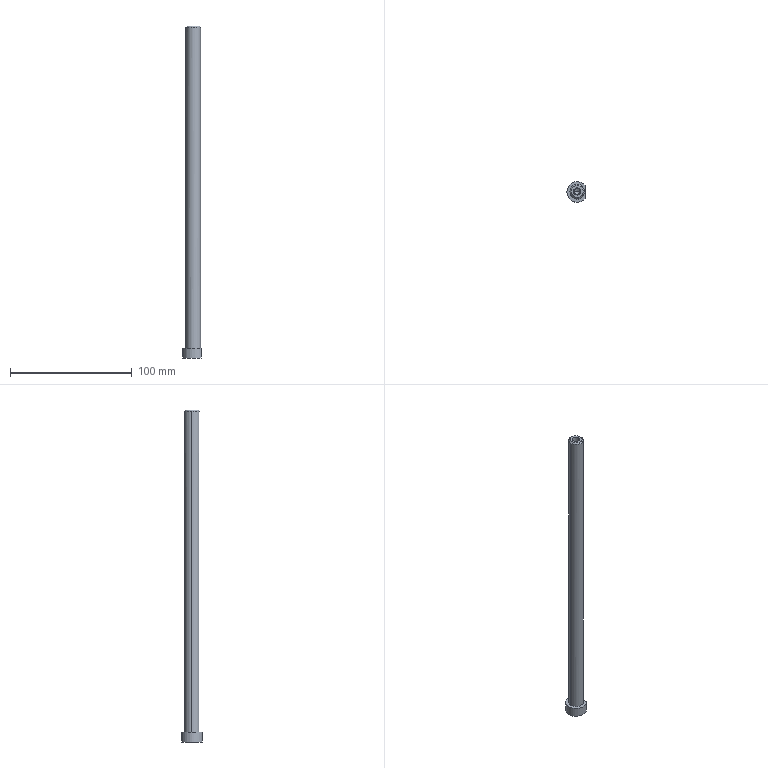Part | Creo | 1 solid | 16 faces | box 15 x 17 x 273 mm | volume 31161 mm3 | cylinder 7 | plane 5 | cone 4 | commonest cylinder face diameters 5 x2 6 x2 12 x2 17 x1
STEP:
#1=CARTESIAN_POINT('',(31.5,12.523,-288.));
#2=VERTEX_POINT('',#1);
#3=CARTESIAN_POINT('',(31.5,23.477,-288.));
#4=VERTEX_POINT('',#3);
#5=CARTESIAN_POINT('',(31.5,12.523,-288.));
#6=DIRECTION('',(0.,1.,0.));
#7=VECTOR('',#6,10.954);
#8=LINE('',#5,#7);
#9=EDGE_CURVE('',#2,#4,#8,.T.);
#10=ORIENTED_EDGE('',*,*,#9,.F.);
#11=CARTESIAN_POINT('',(25.,18.,-288.));
#12=DIRECTION('',(0.,0.,1.));
#13=DIRECTION('',(0.7647,0.6444,0.));
#14=AXIS2_PLACEMENT_3D('',#11,#12,#13);
#15=CIRCLE('',#14,8.5);
#16=EDGE_CURVE('',#4,#2,#15,.T.);
#17=ORIENTED_EDGE('',*,*,#16,.F.);
#18=EDGE_LOOP('',(#10,#17));
#19=FACE_OUTER_BOUND('',#18,.F.);
#20=CARTESIAN_POINT('',(19.,18.,-288.));
#21=VERTEX_POINT('',#20);
#22=CARTESIAN_POINT('',(31.,18.,-288.));
#23=VERTEX_POINT('',#22);
#24=CARTESIAN_POINT('',(25.,18.,-288.));
#25=DIRECTION('',(0.,0.,-1.));
#26=DIRECTION('',(-1.,0.,0.));
#27=AXIS2_PLACEMENT_3D('',#24,#25,#26);
#28=CIRCLE('',#27,6.);
#29=EDGE_CURVE('',#21,#23,#28,.T.);
#30=ORIENTED_EDGE('',*,*,#29,.F.);
#31=CARTESIAN_POINT('',(25.,18.,-288.));
#32=DIRECTION('',(0.,0.,-1.));
#33=DIRECTION('',(1.,0.,0.));
#34=AXIS2_PLACEMENT_3D('',#31,#32,#33);
#35=CIRCLE('',#34,6.);
#36=EDGE_CURVE('',#23,#21,#35,.T.);
#37=ORIENTED_EDGE('',*,*,#36,.F.);
#38=EDGE_LOOP('',(#30,#37));
#39=FACE_BOUND('',#38,.F.);
#40=CARTESIAN_POINT('',(25.,18.,-288.));
#41=DIRECTION('',(0.,0.,1.));
#42=DIRECTION('',(-1.,0.,0.));
#43=AXIS2_PLACEMENT_3D('',#40,#41,#42);
#44=PLANE('',#43);
#45=ADVANCED_FACE('',(#19,#39),#44,.T.);
#46=CARTESIAN_POINT('',(31.5,12.523,-296.));
#47=VERTEX_POINT('',#46);
#48=CARTESIAN_POINT('',(31.5,12.523,-296.));
#49=DIRECTION('',(0.,0.,1.));
#50=VECTOR('',#49,8.);
#51=LINE('',#48,#50);
#52=EDGE_CURVE('',#47,#2,#51,.T.);
#53=ORIENTED_EDGE('',*,*,#52,.T.);
#54=ORIENTED_EDGE('',*,*,#9,.T.);
#55=CARTESIAN_POINT('',(31.5,23.477,-296.));
#56=VERTEX_POINT('',#55);
#57=CARTESIAN_POINT('',(31.5,23.477,-288.));
#58=DIRECTION('',(0.,0.,-1.));
#59=VECTOR('',#58,8.);
#60=LINE('',#57,#59);
#61=EDGE_CURVE('',#4,#56,#60,.T.);
#62=ORIENTED_EDGE('',*,*,#61,.T.);
#63=CARTESIAN_POINT('',(31.5,23.477,-296.));
#64=DIRECTION('',(0.,-1.,0.));
#65=VECTOR('',#64,10.954);
#66=LINE('',#63,#65);
#67=EDGE_CURVE('',#56,#47,#66,.T.);
#68=ORIENTED_EDGE('',*,*,#67,.T.);
#69=EDGE_LOOP('',(#53,#54,#62,#68));
#70=FACE_OUTER_BOUND('',#69,.F.);
#71=CARTESIAN_POINT('',(31.5,53.,-297.));
#72=DIRECTION('',(-1.,0.,0.));
#73=DIRECTION('',(0.,0.,-1.));
#74=AXIS2_PLACEMENT_3D('',#71,#72,#73);
#75=PLANE('',#74);
#76=ADVANCED_FACE('',(#70),#75,.F.);
#77=ORIENTED_EDGE('',*,*,#52,.F.);
#78=CARTESIAN_POINT('',(25.,18.,-296.));
#79=DIRECTION('',(0.,0.,-1.));
#80=DIRECTION('',(0.7647,-0.6444,0.));
#81=AXIS2_PLACEMENT_3D('',#78,#79,#80);
#82=CIRCLE('',#81,8.5);
#83=EDGE_CURVE('',#47,#56,#82,.T.);
#84=ORIENTED_EDGE('',*,*,#83,.T.);
#85=ORIENTED_EDGE('',*,*,#61,.F.);
#86=ORIENTED_EDGE('',*,*,#16,.T.);
#87=EDGE_LOOP('',(#77,#84,#85,#86));
#88=FACE_OUTER_BOUND('',#87,.F.);
#89=CARTESIAN_POINT('',(25.,18.,-296.));
#90=DIRECTION('',(0.,0.,1.));
#91=DIRECTION('',(-1.,0.,0.));
#92=AXIS2_PLACEMENT_3D('',#89,#90,#91);
#93=CYLINDRICAL_SURFACE('',#92,8.5);
#94=ADVANCED_FACE('',(#88),#93,.T.);
#95=ORIENTED_EDGE('',*,*,#67,.F.);
#96=ORIENTED_EDGE('',*,*,#83,.F.);
#97=EDGE_LOOP('',(#95,#96));
#98=FACE_OUTER_BOUND('',#97,.F.);
#99=CARTESIAN_POINT('',(25.,18.,-296.));
#100=DIRECTION('',(0.,0.,-1.));
#101=DIRECTION('',(1.,0.,0.));
#102=AXIS2_PLACEMENT_3D('',#99,#100,#101);
#103=PLANE('',#102);
#104=ADVANCED_FACE('',(#98),#103,.T.);
#105=CARTESIAN_POINT('',(25.,24.,-24.));
#106=VERTEX_POINT('',#105);
#107=CARTESIAN_POINT('',(19.,18.,-24.));
#108=VERTEX_POINT('',#107);
#109=CARTESIAN_POINT('',(25.,18.,-24.));
#110=DIRECTION('',(0.,0.,1.));
#111=DIRECTION('',(0.,1.,0.));
#112=AXIS2_PLACEMENT_3D('',#109,#110,#111);
#113=CIRCLE('',#112,6.);
#114=EDGE_CURVE('',#106,#108,#113,.T.);
#115=ORIENTED_EDGE('',*,*,#114,.T.);
#116=CARTESIAN_POINT('',(19.,18.,-288.));
#117=DIRECTION('',(0.,0.,1.));
#118=VECTOR('',#117,264.);
#119=LINE('',#116,#118);
#120=EDGE_CURVE('',#21,#108,#119,.T.);
#121=ORIENTED_EDGE('',*,*,#120,.F.);
#122=ORIENTED_EDGE('',*,*,#29,.T.);
#123=CARTESIAN_POINT('',(31.,18.,-24.));
#124=VERTEX_POINT('',#123);
#125=CARTESIAN_POINT('',(31.,18.,-288.));
#126=DIRECTION('',(0.,0.,1.));
#127=VECTOR('',#126,264.);
#128=LINE('',#125,#127);
#129=EDGE_CURVE('',#23,#124,#128,.T.);
#130=ORIENTED_EDGE('',*,*,#129,.T.);
#131=CARTESIAN_POINT('',(25.,18.,-24.));
#132=DIRECTION('',(0.,0.,1.));
#133=DIRECTION('',(1.,0.,0.));
#134=AXIS2_PLACEMENT_3D('',#131,#132,#133);
#135=CIRCLE('',#134,6.);
#136=EDGE_CURVE('',#124,#106,#135,.T.);
#137=ORIENTED_EDGE('',*,*,#136,.T.);
#138=EDGE_LOOP('',(#115,#121,#122,#130,#137));
#139=FACE_OUTER_BOUND('',#138,.F.);
#140=CARTESIAN_POINT('',(25.,18.,-351.131));
#141=DIRECTION('',(0.,0.,1.));
#142=DIRECTION('',(-1.,0.,0.));
#143=AXIS2_PLACEMENT_3D('',#140,#141,#142);
#144=CYLINDRICAL_SURFACE('',#143,6.);
#145=ADVANCED_FACE('',(#139),#144,.T.);
#146=ORIENTED_EDGE('',*,*,#114,.F.);
#147=CARTESIAN_POINT('',(25.,23.,-23.));
#148=VERTEX_POINT('',#147);
#149=CARTESIAN_POINT('',(25.,23.,-23.));
#150=DIRECTION('',(0.,0.7071,-0.7071));
#151=VECTOR('',#150,1.414);
#152=LINE('',#149,#151);
#153=EDGE_CURVE('',#148,#106,#152,.T.);
#154=ORIENTED_EDGE('',*,*,#153,.F.);
#155=CARTESIAN_POINT('',(25.,13.,-23.));
#156=VERTEX_POINT('',#155);
#157=CARTESIAN_POINT('',(25.,18.,-23.));
#158=DIRECTION('',(0.,0.,1.));
#159=DIRECTION('',(0.,1.,0.));
#160=AXIS2_PLACEMENT_3D('',#157,#158,#159);
#161=CIRCLE('',#160,5.);
#162=EDGE_CURVE('',#148,#156,#161,.T.);
#163=ORIENTED_EDGE('',*,*,#162,.T.);
#164=CARTESIAN_POINT('',(25.,12.,-24.));
#165=VERTEX_POINT('',#164);
#166=CARTESIAN_POINT('',(25.,13.,-23.));
#167=DIRECTION('',(0.,-0.7071,-0.7071));
#168=VECTOR('',#167,1.414);
#169=LINE('',#166,#168);
#170=EDGE_CURVE('',#156,#165,#169,.T.);
#171=ORIENTED_EDGE('',*,*,#170,.T.);
#172=CARTESIAN_POINT('',(25.,18.,-24.));
#173=DIRECTION('',(0.,0.,1.));
#174=DIRECTION('',(-1.,0.,0.));
#175=AXIS2_PLACEMENT_3D('',#172,#173,#174);
#176=CIRCLE('',#175,6.);
#177=EDGE_CURVE('',#108,#165,#176,.T.);
#178=ORIENTED_EDGE('',*,*,#177,.F.);
#179=EDGE_LOOP('',(#146,#154,#163,#171,#178));
#180=FACE_OUTER_BOUND('',#179,.F.);
#181=CARTESIAN_POINT('',(25.,18.,-23.5));
#182=DIRECTION('',(0.,0.,-1.));
#183=DIRECTION('',(0.,1.,0.));
#184=AXIS2_PLACEMENT_3D('',#181,#182,#183);
#185=CONICAL_SURFACE('',#184,5.5,45.);
#186=ADVANCED_FACE('',(#180),#185,.T.);
#187=CARTESIAN_POINT('',(25.,18.,-24.));
#188=DIRECTION('',(0.,0.,1.));
#189=DIRECTION('',(0.,-1.,0.));
#190=AXIS2_PLACEMENT_3D('',#187,#188,#189);
#191=CIRCLE('',#190,6.);
#192=EDGE_CURVE('',#165,#124,#191,.T.);
#193=ORIENTED_EDGE('',*,*,#192,.F.);
#194=ORIENTED_EDGE('',*,*,#170,.F.);
#195=CARTESIAN_POINT('',(25.,18.,-23.));
#196=DIRECTION('',(0.,0.,1.));
#197=DIRECTION('',(0.,-1.,0.));
#198=AXIS2_PLACEMENT_3D('',#195,#196,#197);
#199=CIRCLE('',#198,5.);
#200=EDGE_CURVE('',#156,#148,#199,.T.);
#201=ORIENTED_EDGE('',*,*,#200,.T.);
#202=ORIENTED_EDGE('',*,*,#153,.T.);
#203=ORIENTED_EDGE('',*,*,#136,.F.);
#204=EDGE_LOOP('',(#193,#194,#201,#202,#203));
#205=FACE_OUTER_BOUND('',#204,.F.);
#206=CARTESIAN_POINT('',(25.,18.,-23.5));
#207=DIRECTION('',(0.,0.,-1.));
#208=DIRECTION('',(0.,1.,0.));
#209=AXIS2_PLACEMENT_3D('',#206,#207,#208);
#210=CONICAL_SURFACE('',#209,5.5,45.);
#211=ADVANCED_FACE('',(#205),#210,.T.);
#212=ORIENTED_EDGE('',*,*,#177,.T.);
#213=ORIENTED_EDGE('',*,*,#192,.T.);
#214=ORIENTED_EDGE('',*,*,#129,.F.);
#215=ORIENTED_EDGE('',*,*,#36,.T.);
#216=ORIENTED_EDGE('',*,*,#120,.T.);
#217=EDGE_LOOP('',(#212,#213,#214,#215,#216));
#218=FACE_OUTER_BOUND('',#217,.F.);
#219=CARTESIAN_POINT('',(25.,18.,-351.131));
#220=DIRECTION('',(0.,0.,1.));
#221=DIRECTION('',(-1.,0.,0.));
#222=AXIS2_PLACEMENT_3D('',#219,#220,#221);
#223=CYLINDRICAL_SURFACE('',#222,6.);
#224=ADVANCED_FACE('',(#218),#223,.T.);
#225=ORIENTED_EDGE('',*,*,#200,.F.);
#226=ORIENTED_EDGE('',*,*,#162,.F.);
#227=EDGE_LOOP('',(#225,#226));
#228=FACE_OUTER_BOUND('',#227,.F.);
#229=CARTESIAN_POINT('',(25.,15.,-23.));
#230=VERTEX_POINT('',#229);
#231=CARTESIAN_POINT('',(22.,18.,-23.));
#232=VERTEX_POINT('',#231);
#233=CARTESIAN_POINT('',(25.,18.,-23.));
#234=DIRECTION('',(0.,0.,-1.));
#235=DIRECTION('',(0.,-1.,0.));
#236=AXIS2_PLACEMENT_3D('',#233,#234,#235);
#237=CIRCLE('',#236,3.);
#238=EDGE_CURVE('',#230,#232,#237,.T.);
#239=ORIENTED_EDGE('',*,*,#238,.F.);
#240=CARTESIAN_POINT('',(28.,18.,-23.));
#241=VERTEX_POINT('',#240);
#242=CARTESIAN_POINT('',(25.,18.,-23.));
#243=DIRECTION('',(0.,0.,-1.));
#244=DIRECTION('',(1.,0.,0.));
#245=AXIS2_PLACEMENT_3D('',#242,#243,#244);
#246=CIRCLE('',#245,3.);
#247=EDGE_CURVE('',#241,#230,#246,.T.);
#248=ORIENTED_EDGE('',*,*,#247,.F.);
#249=CARTESIAN_POINT('',(25.,18.,-23.));
#250=DIRECTION('',(0.,0.,-1.));
#251=DIRECTION('',(-1.,0.,0.));
#252=AXIS2_PLACEMENT_3D('',#249,#250,#251);
#253=CIRCLE('',#252,3.);
#254=EDGE_CURVE('',#232,#241,#253,.T.);
#255=ORIENTED_EDGE('',*,*,#254,.F.);
#256=EDGE_LOOP('',(#239,#248,#255));
#257=FACE_BOUND('',#256,.F.);
#258=CARTESIAN_POINT('',(-50.,35.,-23.));
#259=DIRECTION('',(0.,0.,1.));
#260=DIRECTION('',(-1.,0.,0.));
#261=AXIS2_PLACEMENT_3D('',#258,#259,#260);
#262=PLANE('',#261);
#263=ADVANCED_FACE('',(#228,#257),#262,.T.);
#264=CARTESIAN_POINT('',(22.,18.,-38.872));
#265=VERTEX_POINT('',#264);
#266=CARTESIAN_POINT('',(28.,18.,-38.872));
#267=VERTEX_POINT('',#266);
#268=CARTESIAN_POINT('',(25.,18.,-38.872));
#269=DIRECTION('',(0.,0.,1.));
#270=DIRECTION('',(-1.,0.,0.));
#271=AXIS2_PLACEMENT_3D('',#268,#269,#270);
#272=CIRCLE('',#271,3.);
#273=EDGE_CURVE('',#265,#267,#272,.T.);
#274=ORIENTED_EDGE('',*,*,#273,.T.);
#275=CARTESIAN_POINT('',(28.,18.,-23.));
#276=DIRECTION('',(0.,0.,-1.));
#277=VECTOR('',#276,15.872);
#278=LINE('',#275,#277);
#279=EDGE_CURVE('',#241,#267,#278,.T.);
#280=ORIENTED_EDGE('',*,*,#279,.F.);
#281=ORIENTED_EDGE('',*,*,#247,.T.);
#282=ORIENTED_EDGE('',*,*,#238,.T.);
#283=CARTESIAN_POINT('',(22.,18.,-23.));
#284=DIRECTION('',(0.,0.,-1.));
#285=VECTOR('',#284,15.872);
#286=LINE('',#283,#285);
#287=EDGE_CURVE('',#232,#265,#286,.T.);
#288=ORIENTED_EDGE('',*,*,#287,.T.);
#289=EDGE_LOOP('',(#274,#280,#281,#282,#288));
#290=FACE_OUTER_BOUND('',#289,.F.);
#291=CARTESIAN_POINT('',(25.,18.,-16.372));
#292=DIRECTION('',(0.,0.,-1.));
#293=DIRECTION('',(1.,0.,0.));
#294=AXIS2_PLACEMENT_3D('',#291,#292,#293);
#295=CYLINDRICAL_SURFACE('',#294,3.);
#296=ADVANCED_FACE('',(#290),#295,.F.);
#297=CARTESIAN_POINT('',(25.,18.,-38.872));
#298=DIRECTION('',(0.,0.,1.));
#299=DIRECTION('',(1.,0.,0.));
#300=AXIS2_PLACEMENT_3D('',#297,#298,#299);
#301=CIRCLE('',#300,3.);
#302=EDGE_CURVE('',#267,#265,#301,.T.);
#303=ORIENTED_EDGE('',*,*,#302,.F.);
#304=ORIENTED_EDGE('',*,*,#273,.F.);
#305=EDGE_LOOP('',(#303,#304));
#306=FACE_OUTER_BOUND('',#305,.F.);
#307=CARTESIAN_POINT('',(27.5,18.,-38.872));
#308=VERTEX_POINT('',#307);
#309=CARTESIAN_POINT('',(22.5,18.,-38.872));
#310=VERTEX_POINT('',#309);
#311=CARTESIAN_POINT('',(25.,18.,-38.872));
#312=DIRECTION('',(0.,0.,-1.));
#313=DIRECTION('',(1.,0.,0.));
#314=AXIS2_PLACEMENT_3D('',#311,#312,#313);
#315=CIRCLE('',#314,2.5);
#316=EDGE_CURVE('',#308,#310,#315,.T.);
#317=ORIENTED_EDGE('',*,*,#316,.F.);
#318=CARTESIAN_POINT('',(25.,18.,-38.872));
#319=DIRECTION('',(0.,0.,-1.));
#320=DIRECTION('',(-1.,0.,0.));
#321=AXIS2_PLACEMENT_3D('',#318,#319,#320);
#322=CIRCLE('',#321,2.5);
#323=EDGE_CURVE('',#310,#308,#322,.T.);
#324=ORIENTED_EDGE('',*,*,#323,.F.);
#325=EDGE_LOOP('',(#317,#324));
#326=FACE_BOUND('',#325,.F.);
#327=CARTESIAN_POINT('',(25.,18.,-38.872));
#328=DIRECTION('',(0.,0.,-1.));
#329=DIRECTION('',(1.,0.,0.));
#330=AXIS2_PLACEMENT_3D('',#327,#328,#329);
#331=PLANE('',#330);
#332=ADVANCED_FACE('',(#306,#326),#331,.F.);
#333=ORIENTED_EDGE('',*,*,#316,.T.);
#334=CARTESIAN_POINT('',(22.5,18.,-40.342));
#335=VERTEX_POINT('',#334);
#336=CARTESIAN_POINT('',(22.5,18.,-38.872));
#337=DIRECTION('',(0.,0.,-1.));
#338=VECTOR('',#337,1.47);
#339=LINE('',#336,#338);
#340=EDGE_CURVE('',#310,#335,#339,.T.);
#341=ORIENTED_EDGE('',*,*,#340,.T.);
#342=CARTESIAN_POINT('',(27.5,18.,-40.342));
#343=VERTEX_POINT('',#342);
#344=CARTESIAN_POINT('',(25.,18.,-40.342));
#345=DIRECTION('',(0.,0.,1.));
#346=DIRECTION('',(-1.,0.,0.));
#347=AXIS2_PLACEMENT_3D('',#344,#345,#346);
#348=CIRCLE('',#347,2.5);
#349=EDGE_CURVE('',#335,#343,#348,.T.);
#350=ORIENTED_EDGE('',*,*,#349,.T.);
#351=CARTESIAN_POINT('',(27.5,18.,-38.872));
#352=DIRECTION('',(0.,0.,-1.));
#353=VECTOR('',#352,1.47);
#354=LINE('',#351,#353);
#355=EDGE_CURVE('',#308,#343,#354,.T.);
#356=ORIENTED_EDGE('',*,*,#355,.F.);
#357=EDGE_LOOP('',(#333,#341,#350,#356));
#358=FACE_OUTER_BOUND('',#357,.F.);
#359=CARTESIAN_POINT('',(25.,18.,-16.372));
#360=DIRECTION('',(0.,0.,-1.));
#361=DIRECTION('',(1.,0.,0.));
#362=AXIS2_PLACEMENT_3D('',#359,#360,#361);
#363=CYLINDRICAL_SURFACE('',#362,2.5);
#364=ADVANCED_FACE('',(#358),#363,.F.);
#365=ORIENTED_EDGE('',*,*,#323,.T.);
#366=ORIENTED_EDGE('',*,*,#355,.T.);
#367=CARTESIAN_POINT('',(25.,20.5,-40.342));
#368=VERTEX_POINT('',#367);
#369=CARTESIAN_POINT('',(25.,18.,-40.342));
#370=DIRECTION('',(0.,0.,1.));
#371=DIRECTION('',(1.,0.,0.));
#372=AXIS2_PLACEMENT_3D('',#369,#370,#371);
#373=CIRCLE('',#372,2.5);
#374=EDGE_CURVE('',#343,#368,#373,.T.);
#375=ORIENTED_EDGE('',*,*,#374,.T.);
#376=CARTESIAN_POINT('',(25.,18.,-40.342));
#377=DIRECTION('',(0.,0.,1.));
#378=DIRECTION('',(0.,1.,0.));
#379=AXIS2_PLACEMENT_3D('',#376,#377,#378);
#380=CIRCLE('',#379,2.5);
#381=EDGE_CURVE('',#368,#335,#380,.T.);
#382=ORIENTED_EDGE('',*,*,#381,.T.);
#383=ORIENTED_EDGE('',*,*,#340,.F.);
#384=EDGE_LOOP('',(#365,#366,#375,#382,#383));
#385=FACE_OUTER_BOUND('',#384,.F.);
#386=CARTESIAN_POINT('',(25.,18.,-16.372));
#387=DIRECTION('',(0.,0.,-1.));
#388=DIRECTION('',(1.,0.,0.));
#389=AXIS2_PLACEMENT_3D('',#386,#387,#388);
#390=CYLINDRICAL_SURFACE('',#389,2.5);
#391=ADVANCED_FACE('',(#385),#390,.F.);
#392=ORIENTED_EDGE('',*,*,#381,.F.);
#393=ORIENTED_EDGE('',*,*,#374,.F.);
#394=CARTESIAN_POINT('',(25.,18.,-41.844));
#395=VERTEX_POINT('',#394);
#396=CARTESIAN_POINT('',(25.,18.,-41.844));
#397=DIRECTION('',(0.8572,0.,0.515));
#398=VECTOR('',#397,2.917);
#399=LINE('',#396,#398);
#400=EDGE_CURVE('',#395,#343,#399,.T.);
#401=ORIENTED_EDGE('',*,*,#400,.F.);
#402=CARTESIAN_POINT('',(25.,18.,-41.844));
#403=DIRECTION('',(-0.8572,0.,0.515));
#404=VECTOR('',#403,2.917);
#405=LINE('',#402,#404);
#406=EDGE_CURVE('',#395,#335,#405,.T.);
#407=ORIENTED_EDGE('',*,*,#406,.T.);
#408=EDGE_LOOP('',(#392,#393,#401,#407));
#409=FACE_OUTER_BOUND('',#408,.F.);
#410=CARTESIAN_POINT('',(25.,18.,-41.008));
#411=DIRECTION('',(0.,0.,1.));
#412=DIRECTION('',(1.,0.,0.));
#413=AXIS2_PLACEMENT_3D('',#410,#411,#412);
#414=CONICAL_SURFACE('',#413,1.391,59.);
#415=ADVANCED_FACE('',(#409),#414,.F.);
#416=ORIENTED_EDGE('',*,*,#349,.F.);
#417=ORIENTED_EDGE('',*,*,#406,.F.);
#418=ORIENTED_EDGE('',*,*,#400,.T.);
#419=EDGE_LOOP('',(#416,#417,#418));
#420=FACE_OUTER_BOUND('',#419,.F.);
#421=CARTESIAN_POINT('',(25.,18.,-41.008));
#422=DIRECTION('',(0.,0.,1.));
#423=DIRECTION('',(1.,0.,0.));
#424=AXIS2_PLACEMENT_3D('',#421,#422,#423);
#425=CONICAL_SURFACE('',#424,1.391,59.);
#426=ADVANCED_FACE('',(#420),#425,.F.);
#427=ORIENTED_EDGE('',*,*,#302,.T.);
#428=ORIENTED_EDGE('',*,*,#287,.F.);
#429=ORIENTED_EDGE('',*,*,#254,.T.);
#430=ORIENTED_EDGE('',*,*,#279,.T.);
#431=EDGE_LOOP('',(#427,#428,#429,#430));
#432=FACE_OUTER_BOUND('',#431,.F.);
#433=CARTESIAN_POINT('',(25.,18.,-16.372));
#434=DIRECTION('',(0.,0.,-1.));
#435=DIRECTION('',(1.,0.,0.));
#436=AXIS2_PLACEMENT_3D('',#433,#434,#435);
#437=CYLINDRICAL_SURFACE('',#436,3.);
#438=ADVANCED_FACE('',(#432),#437,.F.);
#439=CLOSED_SHELL('',(#45,#76,#94,#104,#145,#186,#211,#224,#263,#296,#332,#364,#391,#415,#426,#438));
#440=MANIFOLD_SOLID_BREP('',#439);
#441=(LENGTH_UNIT()NAMED_UNIT(*)SI_UNIT(.MILLI.,.METRE.));
#442=UNCERTAINTY_MEASURE_WITH_UNIT(LENGTH_MEASURE(0.02739),#441,'','');
#443=(NAMED_UNIT(*)PLANE_ANGLE_UNIT()SI_UNIT($,.RADIAN.));
#444=PLANE_ANGLE_MEASURE_WITH_UNIT(PLANE_ANGLE_MEASURE(0.01745),#443);
#445=(CONVERSION_BASED_UNIT('DEGREE',#444)NAMED_UNIT(*)PLANE_ANGLE_UNIT());
#446=(NAMED_UNIT(*)SI_UNIT($,.STERADIAN.)SOLID_ANGLE_UNIT());
#447=(GEOMETRIC_REPRESENTATION_CONTEXT(3)GLOBAL_UNCERTAINTY_ASSIGNED_CONTEXT((#442))GLOBAL_UNIT_ASSIGNED_CONTEXT((#441,#445,#446))REPRESENTATION_CONTEXT('',''));
#448=ADVANCED_BREP_SHAPE_REPRESENTATION('',(#440),#447);